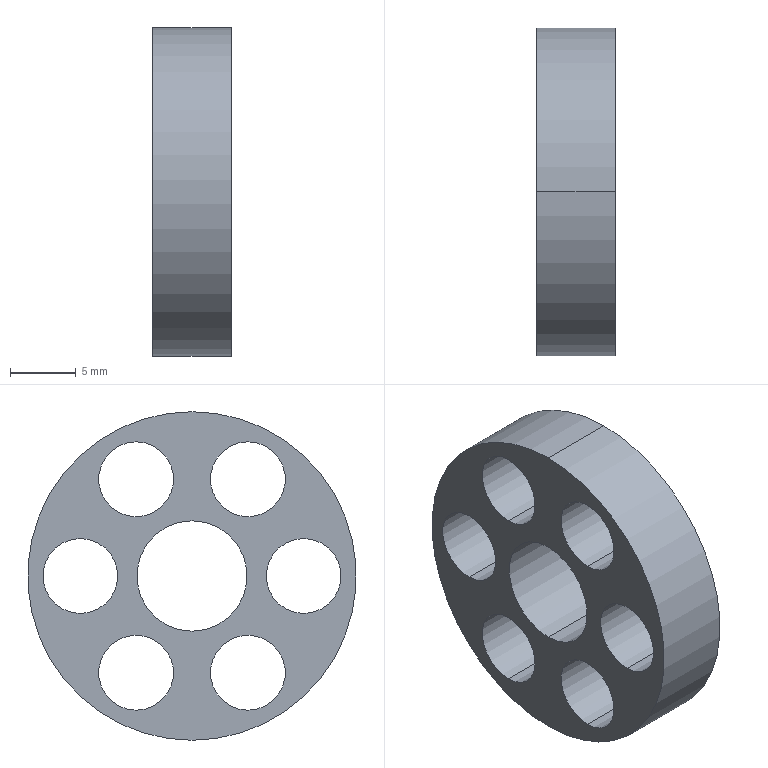Part | SolidWorks | features BaseBody 1 | 1 solid | 18 faces | box 6 x 25 x 25 mm | volume 1694 mm3 | cylinder 16 | plane 2 | commonest cylinder face diameters 5.7 x12 8.4 x2 25 x2
STEP:
#1=CARTESIAN_POINT('',(-3.,0.,-12.5));
#2=VERTEX_POINT('',#1);
#3=CARTESIAN_POINT('',(-3.,0.,12.5));
#4=VERTEX_POINT('',#3);
#5=CARTESIAN_POINT('',(-3.,0.,0.));
#6=DIRECTION('',(1.,0.,0.));
#7=DIRECTION('',(0.,0.,-1.));
#8=AXIS2_PLACEMENT_3D('',#5,#6,#7);
#9=CIRCLE('',#8,12.5);
#10=EDGE_CURVE('',#2,#4,#9,.T.);
#11=ORIENTED_EDGE('',*,*,#10,.T.);
#12=CARTESIAN_POINT('',(3.,0.,12.5));
#13=VERTEX_POINT('',#12);
#14=CARTESIAN_POINT('',(-3.,0.,12.5));
#15=DIRECTION('',(1.,0.,0.));
#16=VECTOR('',#15,1000.);
#17=LINE('',#14,#16);
#18=EDGE_CURVE('',#4,#13,#17,.T.);
#19=ORIENTED_EDGE('',*,*,#18,.T.);
#20=CARTESIAN_POINT('',(3.,0.,-12.5));
#21=VERTEX_POINT('',#20);
#22=CARTESIAN_POINT('',(3.,0.,0.));
#23=DIRECTION('',(-1.,0.,0.));
#24=DIRECTION('',(0.,0.,-1.));
#25=AXIS2_PLACEMENT_3D('',#22,#23,#24);
#26=CIRCLE('',#25,12.5);
#27=EDGE_CURVE('',#13,#21,#26,.T.);
#28=ORIENTED_EDGE('',*,*,#27,.T.);
#29=CARTESIAN_POINT('',(-3.,0.,-12.5));
#30=DIRECTION('',(1.,0.,0.));
#31=VECTOR('',#30,1000.);
#32=LINE('',#29,#31);
#33=EDGE_CURVE('',#2,#21,#32,.T.);
#34=ORIENTED_EDGE('',*,*,#33,.F.);
#35=EDGE_LOOP('',(#11,#19,#28,#34));
#36=FACE_OUTER_BOUND('',#35,.T.);
#37=CARTESIAN_POINT('',(-3.,0.,0.));
#38=DIRECTION('',(1.,0.,0.));
#39=DIRECTION('',(0.,0.,-1.));
#40=AXIS2_PLACEMENT_3D('',#37,#38,#39);
#41=CYLINDRICAL_SURFACE('',#40,12.5);
#42=ADVANCED_FACE('',(#36),#41,.T.);
#43=CARTESIAN_POINT('',(-3.,8.5,-2.85));
#44=VERTEX_POINT('',#43);
#45=CARTESIAN_POINT('',(-3.,8.5,2.85));
#46=VERTEX_POINT('',#45);
#47=CARTESIAN_POINT('',(-3.,8.5,0.));
#48=DIRECTION('',(-1.,0.,0.));
#49=DIRECTION('',(0.,0.,-1.));
#50=AXIS2_PLACEMENT_3D('',#47,#48,#49);
#51=CIRCLE('',#50,2.85);
#52=EDGE_CURVE('',#44,#46,#51,.T.);
#53=ORIENTED_EDGE('',*,*,#52,.T.);
#54=CARTESIAN_POINT('',(3.,8.5,2.85));
#55=VERTEX_POINT('',#54);
#56=CARTESIAN_POINT('',(-4.,8.5,2.85));
#57=DIRECTION('',(1.,0.,0.));
#58=VECTOR('',#57,1000.);
#59=LINE('',#56,#58);
#60=EDGE_CURVE('',#46,#55,#59,.T.);
#61=ORIENTED_EDGE('',*,*,#60,.T.);
#62=CARTESIAN_POINT('',(3.,8.5,-2.85));
#63=VERTEX_POINT('',#62);
#64=CARTESIAN_POINT('',(3.,8.5,0.));
#65=DIRECTION('',(-1.,0.,0.));
#66=DIRECTION('',(0.,0.,-1.));
#67=AXIS2_PLACEMENT_3D('',#64,#65,#66);
#68=CIRCLE('',#67,2.85);
#69=EDGE_CURVE('',#63,#55,#68,.T.);
#70=ORIENTED_EDGE('',*,*,#69,.F.);
#71=CARTESIAN_POINT('',(-4.,8.5,-2.85));
#72=DIRECTION('',(1.,0.,0.));
#73=VECTOR('',#72,1000.);
#74=LINE('',#71,#73);
#75=EDGE_CURVE('',#44,#63,#74,.T.);
#76=ORIENTED_EDGE('',*,*,#75,.F.);
#77=EDGE_LOOP('',(#53,#61,#70,#76));
#78=FACE_OUTER_BOUND('',#77,.T.);
#79=CARTESIAN_POINT('',(-4.,8.5,0.));
#80=DIRECTION('',(1.,0.,0.));
#81=DIRECTION('',(0.,0.,-1.));
#82=AXIS2_PLACEMENT_3D('',#79,#80,#81);
#83=CYLINDRICAL_SURFACE('',#82,2.85);
#84=ADVANCED_FACE('',(#78),#83,.F.);
#85=CARTESIAN_POINT('',(-3.,4.25,-10.211));
#86=VERTEX_POINT('',#85);
#87=CARTESIAN_POINT('',(-3.,4.25,-4.511));
#88=VERTEX_POINT('',#87);
#89=CARTESIAN_POINT('',(-3.,4.25,-7.361));
#90=DIRECTION('',(-1.,0.,0.));
#91=DIRECTION('',(0.,0.,-1.));
#92=AXIS2_PLACEMENT_3D('',#89,#90,#91);
#93=CIRCLE('',#92,2.85);
#94=EDGE_CURVE('',#86,#88,#93,.T.);
#95=ORIENTED_EDGE('',*,*,#94,.T.);
#96=CARTESIAN_POINT('',(3.,4.25,-4.511));
#97=VERTEX_POINT('',#96);
#98=CARTESIAN_POINT('',(-4.,4.25,-4.511));
#99=DIRECTION('',(1.,0.,0.));
#100=VECTOR('',#99,1000.);
#101=LINE('',#98,#100);
#102=EDGE_CURVE('',#88,#97,#101,.T.);
#103=ORIENTED_EDGE('',*,*,#102,.T.);
#104=CARTESIAN_POINT('',(3.,4.25,-10.211));
#105=VERTEX_POINT('',#104);
#106=CARTESIAN_POINT('',(3.,4.25,-7.361));
#107=DIRECTION('',(-1.,0.,0.));
#108=DIRECTION('',(0.,0.,-1.));
#109=AXIS2_PLACEMENT_3D('',#106,#107,#108);
#110=CIRCLE('',#109,2.85);
#111=EDGE_CURVE('',#105,#97,#110,.T.);
#112=ORIENTED_EDGE('',*,*,#111,.F.);
#113=CARTESIAN_POINT('',(-4.,4.25,-10.211));
#114=DIRECTION('',(1.,0.,0.));
#115=VECTOR('',#114,1000.);
#116=LINE('',#113,#115);
#117=EDGE_CURVE('',#86,#105,#116,.T.);
#118=ORIENTED_EDGE('',*,*,#117,.F.);
#119=EDGE_LOOP('',(#95,#103,#112,#118));
#120=FACE_OUTER_BOUND('',#119,.T.);
#121=CARTESIAN_POINT('',(-4.,4.25,-7.361));
#122=DIRECTION('',(1.,0.,0.));
#123=DIRECTION('',(0.,0.,-1.));
#124=AXIS2_PLACEMENT_3D('',#121,#122,#123);
#125=CYLINDRICAL_SURFACE('',#124,2.85);
#126=ADVANCED_FACE('',(#120),#125,.F.);
#127=CARTESIAN_POINT('',(-3.,0.,-4.2));
#128=VERTEX_POINT('',#127);
#129=CARTESIAN_POINT('',(-3.,0.,4.2));
#130=VERTEX_POINT('',#129);
#131=CARTESIAN_POINT('',(-3.,0.,0.));
#132=DIRECTION('',(-1.,0.,0.));
#133=DIRECTION('',(0.,0.,-1.));
#134=AXIS2_PLACEMENT_3D('',#131,#132,#133);
#135=CIRCLE('',#134,4.2);
#136=EDGE_CURVE('',#128,#130,#135,.T.);
#137=ORIENTED_EDGE('',*,*,#136,.T.);
#138=CARTESIAN_POINT('',(3.,0.,4.2));
#139=VERTEX_POINT('',#138);
#140=CARTESIAN_POINT('',(-4.,0.,4.2));
#141=DIRECTION('',(1.,0.,0.));
#142=VECTOR('',#141,1000.);
#143=LINE('',#140,#142);
#144=EDGE_CURVE('',#130,#139,#143,.T.);
#145=ORIENTED_EDGE('',*,*,#144,.T.);
#146=CARTESIAN_POINT('',(3.,0.,-4.2));
#147=VERTEX_POINT('',#146);
#148=CARTESIAN_POINT('',(3.,0.,0.));
#149=DIRECTION('',(-1.,0.,0.));
#150=DIRECTION('',(0.,0.,-1.));
#151=AXIS2_PLACEMENT_3D('',#148,#149,#150);
#152=CIRCLE('',#151,4.2);
#153=EDGE_CURVE('',#147,#139,#152,.T.);
#154=ORIENTED_EDGE('',*,*,#153,.F.);
#155=CARTESIAN_POINT('',(-4.,0.,-4.2));
#156=DIRECTION('',(1.,0.,0.));
#157=VECTOR('',#156,1000.);
#158=LINE('',#155,#157);
#159=EDGE_CURVE('',#128,#147,#158,.T.);
#160=ORIENTED_EDGE('',*,*,#159,.F.);
#161=EDGE_LOOP('',(#137,#145,#154,#160));
#162=FACE_OUTER_BOUND('',#161,.T.);
#163=CARTESIAN_POINT('',(-4.,0.,0.));
#164=DIRECTION('',(1.,0.,0.));
#165=DIRECTION('',(0.,0.,-1.));
#166=AXIS2_PLACEMENT_3D('',#163,#164,#165);
#167=CYLINDRICAL_SURFACE('',#166,4.2);
#168=ADVANCED_FACE('',(#162),#167,.F.);
#169=CARTESIAN_POINT('',(-3.,4.25,4.511));
#170=VERTEX_POINT('',#169);
#171=CARTESIAN_POINT('',(-3.,4.25,10.211));
#172=VERTEX_POINT('',#171);
#173=CARTESIAN_POINT('',(-3.,4.25,7.361));
#174=DIRECTION('',(-1.,0.,0.));
#175=DIRECTION('',(0.,0.,-1.));
#176=AXIS2_PLACEMENT_3D('',#173,#174,#175);
#177=CIRCLE('',#176,2.85);
#178=EDGE_CURVE('',#170,#172,#177,.T.);
#179=ORIENTED_EDGE('',*,*,#178,.T.);
#180=CARTESIAN_POINT('',(3.,4.25,10.211));
#181=VERTEX_POINT('',#180);
#182=CARTESIAN_POINT('',(-4.,4.25,10.211));
#183=DIRECTION('',(1.,0.,0.));
#184=VECTOR('',#183,1000.);
#185=LINE('',#182,#184);
#186=EDGE_CURVE('',#172,#181,#185,.T.);
#187=ORIENTED_EDGE('',*,*,#186,.T.);
#188=CARTESIAN_POINT('',(3.,4.25,4.511));
#189=VERTEX_POINT('',#188);
#190=CARTESIAN_POINT('',(3.,4.25,7.361));
#191=DIRECTION('',(-1.,0.,0.));
#192=DIRECTION('',(0.,0.,-1.));
#193=AXIS2_PLACEMENT_3D('',#190,#191,#192);
#194=CIRCLE('',#193,2.85);
#195=EDGE_CURVE('',#189,#181,#194,.T.);
#196=ORIENTED_EDGE('',*,*,#195,.F.);
#197=CARTESIAN_POINT('',(-4.,4.25,4.511));
#198=DIRECTION('',(1.,0.,0.));
#199=VECTOR('',#198,1000.);
#200=LINE('',#197,#199);
#201=EDGE_CURVE('',#170,#189,#200,.T.);
#202=ORIENTED_EDGE('',*,*,#201,.F.);
#203=EDGE_LOOP('',(#179,#187,#196,#202));
#204=FACE_OUTER_BOUND('',#203,.T.);
#205=CARTESIAN_POINT('',(-4.,4.25,7.361));
#206=DIRECTION('',(1.,0.,0.));
#207=DIRECTION('',(0.,0.,-1.));
#208=AXIS2_PLACEMENT_3D('',#205,#206,#207);
#209=CYLINDRICAL_SURFACE('',#208,2.85);
#210=ADVANCED_FACE('',(#204),#209,.F.);
#211=CARTESIAN_POINT('',(-3.,-4.25,-10.211));
#212=VERTEX_POINT('',#211);
#213=CARTESIAN_POINT('',(-3.,-4.25,-4.511));
#214=VERTEX_POINT('',#213);
#215=CARTESIAN_POINT('',(-3.,-4.25,-7.361));
#216=DIRECTION('',(-1.,0.,0.));
#217=DIRECTION('',(0.,0.,-1.));
#218=AXIS2_PLACEMENT_3D('',#215,#216,#217);
#219=CIRCLE('',#218,2.85);
#220=EDGE_CURVE('',#212,#214,#219,.T.);
#221=ORIENTED_EDGE('',*,*,#220,.T.);
#222=CARTESIAN_POINT('',(3.,-4.25,-4.511));
#223=VERTEX_POINT('',#222);
#224=CARTESIAN_POINT('',(-4.,-4.25,-4.511));
#225=DIRECTION('',(1.,0.,0.));
#226=VECTOR('',#225,1000.);
#227=LINE('',#224,#226);
#228=EDGE_CURVE('',#214,#223,#227,.T.);
#229=ORIENTED_EDGE('',*,*,#228,.T.);
#230=CARTESIAN_POINT('',(3.,-4.25,-10.211));
#231=VERTEX_POINT('',#230);
#232=CARTESIAN_POINT('',(3.,-4.25,-7.361));
#233=DIRECTION('',(-1.,0.,0.));
#234=DIRECTION('',(0.,0.,-1.));
#235=AXIS2_PLACEMENT_3D('',#232,#233,#234);
#236=CIRCLE('',#235,2.85);
#237=EDGE_CURVE('',#231,#223,#236,.T.);
#238=ORIENTED_EDGE('',*,*,#237,.F.);
#239=CARTESIAN_POINT('',(-4.,-4.25,-10.211));
#240=DIRECTION('',(1.,0.,0.));
#241=VECTOR('',#240,1000.);
#242=LINE('',#239,#241);
#243=EDGE_CURVE('',#212,#231,#242,.T.);
#244=ORIENTED_EDGE('',*,*,#243,.F.);
#245=EDGE_LOOP('',(#221,#229,#238,#244));
#246=FACE_OUTER_BOUND('',#245,.T.);
#247=CARTESIAN_POINT('',(-4.,-4.25,-7.361));
#248=DIRECTION('',(1.,0.,0.));
#249=DIRECTION('',(0.,0.,-1.));
#250=AXIS2_PLACEMENT_3D('',#247,#248,#249);
#251=CYLINDRICAL_SURFACE('',#250,2.85);
#252=ADVANCED_FACE('',(#246),#251,.F.);
#253=CARTESIAN_POINT('',(-3.,-8.5,-2.85));
#254=VERTEX_POINT('',#253);
#255=CARTESIAN_POINT('',(-3.,-8.5,2.85));
#256=VERTEX_POINT('',#255);
#257=CARTESIAN_POINT('',(-3.,-8.5,0.));
#258=DIRECTION('',(-1.,0.,0.));
#259=DIRECTION('',(0.,0.,-1.));
#260=AXIS2_PLACEMENT_3D('',#257,#258,#259);
#261=CIRCLE('',#260,2.85);
#262=EDGE_CURVE('',#254,#256,#261,.T.);
#263=ORIENTED_EDGE('',*,*,#262,.T.);
#264=CARTESIAN_POINT('',(3.,-8.5,2.85));
#265=VERTEX_POINT('',#264);
#266=CARTESIAN_POINT('',(-4.,-8.5,2.85));
#267=DIRECTION('',(1.,0.,0.));
#268=VECTOR('',#267,1000.);
#269=LINE('',#266,#268);
#270=EDGE_CURVE('',#256,#265,#269,.T.);
#271=ORIENTED_EDGE('',*,*,#270,.T.);
#272=CARTESIAN_POINT('',(3.,-8.5,-2.85));
#273=VERTEX_POINT('',#272);
#274=CARTESIAN_POINT('',(3.,-8.5,0.));
#275=DIRECTION('',(-1.,0.,0.));
#276=DIRECTION('',(0.,0.,-1.));
#277=AXIS2_PLACEMENT_3D('',#274,#275,#276);
#278=CIRCLE('',#277,2.85);
#279=EDGE_CURVE('',#273,#265,#278,.T.);
#280=ORIENTED_EDGE('',*,*,#279,.F.);
#281=CARTESIAN_POINT('',(-4.,-8.5,-2.85));
#282=DIRECTION('',(1.,0.,0.));
#283=VECTOR('',#282,1000.);
#284=LINE('',#281,#283);
#285=EDGE_CURVE('',#254,#273,#284,.T.);
#286=ORIENTED_EDGE('',*,*,#285,.F.);
#287=EDGE_LOOP('',(#263,#271,#280,#286));
#288=FACE_OUTER_BOUND('',#287,.T.);
#289=CARTESIAN_POINT('',(-4.,-8.5,0.));
#290=DIRECTION('',(1.,0.,0.));
#291=DIRECTION('',(0.,0.,-1.));
#292=AXIS2_PLACEMENT_3D('',#289,#290,#291);
#293=CYLINDRICAL_SURFACE('',#292,2.85);
#294=ADVANCED_FACE('',(#288),#293,.F.);
#295=CARTESIAN_POINT('',(-3.,-4.25,4.511));
#296=VERTEX_POINT('',#295);
#297=CARTESIAN_POINT('',(-3.,-4.25,10.211));
#298=VERTEX_POINT('',#297);
#299=CARTESIAN_POINT('',(-3.,-4.25,7.361));
#300=DIRECTION('',(-1.,0.,0.));
#301=DIRECTION('',(0.,0.,-1.));
#302=AXIS2_PLACEMENT_3D('',#299,#300,#301);
#303=CIRCLE('',#302,2.85);
#304=EDGE_CURVE('',#296,#298,#303,.T.);
#305=ORIENTED_EDGE('',*,*,#304,.T.);
#306=CARTESIAN_POINT('',(3.,-4.25,10.211));
#307=VERTEX_POINT('',#306);
#308=CARTESIAN_POINT('',(-4.,-4.25,10.211));
#309=DIRECTION('',(1.,0.,0.));
#310=VECTOR('',#309,1000.);
#311=LINE('',#308,#310);
#312=EDGE_CURVE('',#298,#307,#311,.T.);
#313=ORIENTED_EDGE('',*,*,#312,.T.);
#314=CARTESIAN_POINT('',(3.,-4.25,4.511));
#315=VERTEX_POINT('',#314);
#316=CARTESIAN_POINT('',(3.,-4.25,7.361));
#317=DIRECTION('',(-1.,0.,0.));
#318=DIRECTION('',(0.,0.,-1.));
#319=AXIS2_PLACEMENT_3D('',#316,#317,#318);
#320=CIRCLE('',#319,2.85);
#321=EDGE_CURVE('',#315,#307,#320,.T.);
#322=ORIENTED_EDGE('',*,*,#321,.F.);
#323=CARTESIAN_POINT('',(-4.,-4.25,4.511));
#324=DIRECTION('',(1.,0.,0.));
#325=VECTOR('',#324,1000.);
#326=LINE('',#323,#325);
#327=EDGE_CURVE('',#296,#315,#326,.T.);
#328=ORIENTED_EDGE('',*,*,#327,.F.);
#329=EDGE_LOOP('',(#305,#313,#322,#328));
#330=FACE_OUTER_BOUND('',#329,.T.);
#331=CARTESIAN_POINT('',(-4.,-4.25,7.361));
#332=DIRECTION('',(1.,0.,0.));
#333=DIRECTION('',(0.,0.,-1.));
#334=AXIS2_PLACEMENT_3D('',#331,#332,#333);
#335=CYLINDRICAL_SURFACE('',#334,2.85);
#336=ADVANCED_FACE('',(#330),#335,.F.);
#337=ORIENTED_EDGE('',*,*,#18,.F.);
#338=CARTESIAN_POINT('',(-3.,0.,0.));
#339=DIRECTION('',(1.,0.,0.));
#340=DIRECTION('',(0.,0.,-1.));
#341=AXIS2_PLACEMENT_3D('',#338,#339,#340);
#342=CIRCLE('',#341,12.5);
#343=EDGE_CURVE('',#4,#2,#342,.T.);
#344=ORIENTED_EDGE('',*,*,#343,.T.);
#345=ORIENTED_EDGE('',*,*,#33,.T.);
#346=CARTESIAN_POINT('',(3.,0.,0.));
#347=DIRECTION('',(-1.,0.,0.));
#348=DIRECTION('',(0.,0.,-1.));
#349=AXIS2_PLACEMENT_3D('',#346,#347,#348);
#350=CIRCLE('',#349,12.5);
#351=EDGE_CURVE('',#21,#13,#350,.T.);
#352=ORIENTED_EDGE('',*,*,#351,.T.);
#353=EDGE_LOOP('',(#337,#344,#345,#352));
#354=FACE_OUTER_BOUND('',#353,.T.);
#355=CARTESIAN_POINT('',(-3.,0.,0.));
#356=DIRECTION('',(1.,0.,0.));
#357=DIRECTION('',(0.,0.,-1.));
#358=AXIS2_PLACEMENT_3D('',#355,#356,#357);
#359=CYLINDRICAL_SURFACE('',#358,12.5);
#360=ADVANCED_FACE('',(#354),#359,.T.);
#361=ORIENTED_EDGE('',*,*,#52,.F.);
#362=CARTESIAN_POINT('',(-3.,8.5,0.));
#363=DIRECTION('',(-1.,0.,0.));
#364=DIRECTION('',(0.,0.,-1.));
#365=AXIS2_PLACEMENT_3D('',#362,#363,#364);
#366=CIRCLE('',#365,2.85);
#367=EDGE_CURVE('',#46,#44,#366,.T.);
#368=ORIENTED_EDGE('',*,*,#367,.F.);
#369=EDGE_LOOP('',(#361,#368));
#370=FACE_BOUND('',#369,.T.);
#371=ORIENTED_EDGE('',*,*,#94,.F.);
#372=CARTESIAN_POINT('',(-3.,4.25,-7.361));
#373=DIRECTION('',(-1.,0.,0.));
#374=DIRECTION('',(0.,0.,-1.));
#375=AXIS2_PLACEMENT_3D('',#372,#373,#374);
#376=CIRCLE('',#375,2.85);
#377=EDGE_CURVE('',#88,#86,#376,.T.);
#378=ORIENTED_EDGE('',*,*,#377,.F.);
#379=EDGE_LOOP('',(#371,#378));
#380=FACE_BOUND('',#379,.T.);
#381=ORIENTED_EDGE('',*,*,#136,.F.);
#382=CARTESIAN_POINT('',(-3.,0.,0.));
#383=DIRECTION('',(-1.,0.,0.));
#384=DIRECTION('',(0.,0.,-1.));
#385=AXIS2_PLACEMENT_3D('',#382,#383,#384);
#386=CIRCLE('',#385,4.2);
#387=EDGE_CURVE('',#130,#128,#386,.T.);
#388=ORIENTED_EDGE('',*,*,#387,.F.);
#389=EDGE_LOOP('',(#381,#388));
#390=FACE_BOUND('',#389,.T.);
#391=ORIENTED_EDGE('',*,*,#178,.F.);
#392=CARTESIAN_POINT('',(-3.,4.25,7.361));
#393=DIRECTION('',(-1.,0.,0.));
#394=DIRECTION('',(0.,0.,-1.));
#395=AXIS2_PLACEMENT_3D('',#392,#393,#394);
#396=CIRCLE('',#395,2.85);
#397=EDGE_CURVE('',#172,#170,#396,.T.);
#398=ORIENTED_EDGE('',*,*,#397,.F.);
#399=EDGE_LOOP('',(#391,#398));
#400=FACE_BOUND('',#399,.T.);
#401=ORIENTED_EDGE('',*,*,#220,.F.);
#402=CARTESIAN_POINT('',(-3.,-4.25,-7.361));
#403=DIRECTION('',(-1.,0.,0.));
#404=DIRECTION('',(0.,0.,-1.));
#405=AXIS2_PLACEMENT_3D('',#402,#403,#404);
#406=CIRCLE('',#405,2.85);
#407=EDGE_CURVE('',#214,#212,#406,.T.);
#408=ORIENTED_EDGE('',*,*,#407,.F.);
#409=EDGE_LOOP('',(#401,#408));
#410=FACE_BOUND('',#409,.T.);
#411=ORIENTED_EDGE('',*,*,#262,.F.);
#412=CARTESIAN_POINT('',(-3.,-8.5,0.));
#413=DIRECTION('',(-1.,0.,0.));
#414=DIRECTION('',(0.,0.,-1.));
#415=AXIS2_PLACEMENT_3D('',#412,#413,#414);
#416=CIRCLE('',#415,2.85);
#417=EDGE_CURVE('',#256,#254,#416,.T.);
#418=ORIENTED_EDGE('',*,*,#417,.F.);
#419=EDGE_LOOP('',(#411,#418));
#420=FACE_BOUND('',#419,.T.);
#421=ORIENTED_EDGE('',*,*,#304,.F.);
#422=CARTESIAN_POINT('',(-3.,-4.25,7.361));
#423=DIRECTION('',(-1.,0.,0.));
#424=DIRECTION('',(0.,0.,-1.));
#425=AXIS2_PLACEMENT_3D('',#422,#423,#424);
#426=CIRCLE('',#425,2.85);
#427=EDGE_CURVE('',#298,#296,#426,.T.);
#428=ORIENTED_EDGE('',*,*,#427,.F.);
#429=EDGE_LOOP('',(#421,#428));
#430=FACE_BOUND('',#429,.T.);
#431=ORIENTED_EDGE('',*,*,#10,.F.);
#432=ORIENTED_EDGE('',*,*,#343,.F.);
#433=EDGE_LOOP('',(#431,#432));
#434=FACE_OUTER_BOUND('',#433,.T.);
#435=CARTESIAN_POINT('',(-3.,0.,0.));
#436=DIRECTION('',(1.,0.,0.));
#437=DIRECTION('',(0.,0.,-1.));
#438=AXIS2_PLACEMENT_3D('',#435,#436,#437);
#439=PLANE('',#438);
#440=ADVANCED_FACE('',(#370,#380,#390,#400,#410,#420,#430,#434),#439,.F.);
#441=ORIENTED_EDGE('',*,*,#69,.T.);
#442=CARTESIAN_POINT('',(3.,8.5,0.));
#443=DIRECTION('',(-1.,0.,0.));
#444=DIRECTION('',(0.,0.,-1.));
#445=AXIS2_PLACEMENT_3D('',#442,#443,#444);
#446=CIRCLE('',#445,2.85);
#447=EDGE_CURVE('',#55,#63,#446,.T.);
#448=ORIENTED_EDGE('',*,*,#447,.T.);
#449=EDGE_LOOP('',(#441,#448));
#450=FACE_BOUND('',#449,.T.);
#451=ORIENTED_EDGE('',*,*,#111,.T.);
#452=CARTESIAN_POINT('',(3.,4.25,-7.361));
#453=DIRECTION('',(-1.,0.,0.));
#454=DIRECTION('',(0.,0.,-1.));
#455=AXIS2_PLACEMENT_3D('',#452,#453,#454);
#456=CIRCLE('',#455,2.85);
#457=EDGE_CURVE('',#97,#105,#456,.T.);
#458=ORIENTED_EDGE('',*,*,#457,.T.);
#459=EDGE_LOOP('',(#451,#458));
#460=FACE_BOUND('',#459,.T.);
#461=ORIENTED_EDGE('',*,*,#153,.T.);
#462=CARTESIAN_POINT('',(3.,0.,0.));
#463=DIRECTION('',(-1.,0.,0.));
#464=DIRECTION('',(0.,0.,-1.));
#465=AXIS2_PLACEMENT_3D('',#462,#463,#464);
#466=CIRCLE('',#465,4.2);
#467=EDGE_CURVE('',#139,#147,#466,.T.);
#468=ORIENTED_EDGE('',*,*,#467,.T.);
#469=EDGE_LOOP('',(#461,#468));
#470=FACE_BOUND('',#469,.T.);
#471=ORIENTED_EDGE('',*,*,#195,.T.);
#472=CARTESIAN_POINT('',(3.,4.25,7.361));
#473=DIRECTION('',(-1.,0.,0.));
#474=DIRECTION('',(0.,0.,-1.));
#475=AXIS2_PLACEMENT_3D('',#472,#473,#474);
#476=CIRCLE('',#475,2.85);
#477=EDGE_CURVE('',#181,#189,#476,.T.);
#478=ORIENTED_EDGE('',*,*,#477,.T.);
#479=EDGE_LOOP('',(#471,#478));
#480=FACE_BOUND('',#479,.T.);
#481=ORIENTED_EDGE('',*,*,#237,.T.);
#482=CARTESIAN_POINT('',(3.,-4.25,-7.361));
#483=DIRECTION('',(-1.,0.,0.));
#484=DIRECTION('',(0.,0.,-1.));
#485=AXIS2_PLACEMENT_3D('',#482,#483,#484);
#486=CIRCLE('',#485,2.85);
#487=EDGE_CURVE('',#223,#231,#486,.T.);
#488=ORIENTED_EDGE('',*,*,#487,.T.);
#489=EDGE_LOOP('',(#481,#488));
#490=FACE_BOUND('',#489,.T.);
#491=ORIENTED_EDGE('',*,*,#279,.T.);
#492=CARTESIAN_POINT('',(3.,-8.5,0.));
#493=DIRECTION('',(-1.,0.,0.));
#494=DIRECTION('',(0.,0.,-1.));
#495=AXIS2_PLACEMENT_3D('',#492,#493,#494);
#496=CIRCLE('',#495,2.85);
#497=EDGE_CURVE('',#265,#273,#496,.T.);
#498=ORIENTED_EDGE('',*,*,#497,.T.);
#499=EDGE_LOOP('',(#491,#498));
#500=FACE_BOUND('',#499,.T.);
#501=ORIENTED_EDGE('',*,*,#321,.T.);
#502=CARTESIAN_POINT('',(3.,-4.25,7.361));
#503=DIRECTION('',(-1.,0.,0.));
#504=DIRECTION('',(0.,0.,-1.));
#505=AXIS2_PLACEMENT_3D('',#502,#503,#504);
#506=CIRCLE('',#505,2.85);
#507=EDGE_CURVE('',#307,#315,#506,.T.);
#508=ORIENTED_EDGE('',*,*,#507,.T.);
#509=EDGE_LOOP('',(#501,#508));
#510=FACE_BOUND('',#509,.T.);
#511=ORIENTED_EDGE('',*,*,#351,.F.);
#512=ORIENTED_EDGE('',*,*,#27,.F.);
#513=EDGE_LOOP('',(#511,#512));
#514=FACE_OUTER_BOUND('',#513,.T.);
#515=CARTESIAN_POINT('',(3.,0.,0.));
#516=DIRECTION('',(1.,0.,0.));
#517=DIRECTION('',(0.,0.,-1.));
#518=AXIS2_PLACEMENT_3D('',#515,#516,#517);
#519=PLANE('',#518);
#520=ADVANCED_FACE('',(#450,#460,#470,#480,#490,#500,#510,#514),#519,.T.);
#521=ORIENTED_EDGE('',*,*,#60,.F.);
#522=ORIENTED_EDGE('',*,*,#367,.T.);
#523=ORIENTED_EDGE('',*,*,#75,.T.);
#524=ORIENTED_EDGE('',*,*,#447,.F.);
#525=EDGE_LOOP('',(#521,#522,#523,#524));
#526=FACE_OUTER_BOUND('',#525,.T.);
#527=CARTESIAN_POINT('',(-4.,8.5,0.));
#528=DIRECTION('',(1.,0.,0.));
#529=DIRECTION('',(0.,0.,-1.));
#530=AXIS2_PLACEMENT_3D('',#527,#528,#529);
#531=CYLINDRICAL_SURFACE('',#530,2.85);
#532=ADVANCED_FACE('',(#526),#531,.F.);
#533=ORIENTED_EDGE('',*,*,#102,.F.);
#534=ORIENTED_EDGE('',*,*,#377,.T.);
#535=ORIENTED_EDGE('',*,*,#117,.T.);
#536=ORIENTED_EDGE('',*,*,#457,.F.);
#537=EDGE_LOOP('',(#533,#534,#535,#536));
#538=FACE_OUTER_BOUND('',#537,.T.);
#539=CARTESIAN_POINT('',(-4.,4.25,-7.361));
#540=DIRECTION('',(1.,0.,0.));
#541=DIRECTION('',(0.,0.,-1.));
#542=AXIS2_PLACEMENT_3D('',#539,#540,#541);
#543=CYLINDRICAL_SURFACE('',#542,2.85);
#544=ADVANCED_FACE('',(#538),#543,.F.);
#545=ORIENTED_EDGE('',*,*,#144,.F.);
#546=ORIENTED_EDGE('',*,*,#387,.T.);
#547=ORIENTED_EDGE('',*,*,#159,.T.);
#548=ORIENTED_EDGE('',*,*,#467,.F.);
#549=EDGE_LOOP('',(#545,#546,#547,#548));
#550=FACE_OUTER_BOUND('',#549,.T.);
#551=CARTESIAN_POINT('',(-4.,0.,0.));
#552=DIRECTION('',(1.,0.,0.));
#553=DIRECTION('',(0.,0.,-1.));
#554=AXIS2_PLACEMENT_3D('',#551,#552,#553);
#555=CYLINDRICAL_SURFACE('',#554,4.2);
#556=ADVANCED_FACE('',(#550),#555,.F.);
#557=ORIENTED_EDGE('',*,*,#186,.F.);
#558=ORIENTED_EDGE('',*,*,#397,.T.);
#559=ORIENTED_EDGE('',*,*,#201,.T.);
#560=ORIENTED_EDGE('',*,*,#477,.F.);
#561=EDGE_LOOP('',(#557,#558,#559,#560));
#562=FACE_OUTER_BOUND('',#561,.T.);
#563=CARTESIAN_POINT('',(-4.,4.25,7.361));
#564=DIRECTION('',(1.,0.,0.));
#565=DIRECTION('',(0.,0.,-1.));
#566=AXIS2_PLACEMENT_3D('',#563,#564,#565);
#567=CYLINDRICAL_SURFACE('',#566,2.85);
#568=ADVANCED_FACE('',(#562),#567,.F.);
#569=ORIENTED_EDGE('',*,*,#228,.F.);
#570=ORIENTED_EDGE('',*,*,#407,.T.);
#571=ORIENTED_EDGE('',*,*,#243,.T.);
#572=ORIENTED_EDGE('',*,*,#487,.F.);
#573=EDGE_LOOP('',(#569,#570,#571,#572));
#574=FACE_OUTER_BOUND('',#573,.T.);
#575=CARTESIAN_POINT('',(-4.,-4.25,-7.361));
#576=DIRECTION('',(1.,0.,0.));
#577=DIRECTION('',(0.,0.,-1.));
#578=AXIS2_PLACEMENT_3D('',#575,#576,#577);
#579=CYLINDRICAL_SURFACE('',#578,2.85);
#580=ADVANCED_FACE('',(#574),#579,.F.);
#581=ORIENTED_EDGE('',*,*,#270,.F.);
#582=ORIENTED_EDGE('',*,*,#417,.T.);
#583=ORIENTED_EDGE('',*,*,#285,.T.);
#584=ORIENTED_EDGE('',*,*,#497,.F.);
#585=EDGE_LOOP('',(#581,#582,#583,#584));
#586=FACE_OUTER_BOUND('',#585,.T.);
#587=CARTESIAN_POINT('',(-4.,-8.5,0.));
#588=DIRECTION('',(1.,0.,0.));
#589=DIRECTION('',(0.,0.,-1.));
#590=AXIS2_PLACEMENT_3D('',#587,#588,#589);
#591=CYLINDRICAL_SURFACE('',#590,2.85);
#592=ADVANCED_FACE('',(#586),#591,.F.);
#593=ORIENTED_EDGE('',*,*,#312,.F.);
#594=ORIENTED_EDGE('',*,*,#427,.T.);
#595=ORIENTED_EDGE('',*,*,#327,.T.);
#596=ORIENTED_EDGE('',*,*,#507,.F.);
#597=EDGE_LOOP('',(#593,#594,#595,#596));
#598=FACE_OUTER_BOUND('',#597,.T.);
#599=CARTESIAN_POINT('',(-4.,-4.25,7.361));
#600=DIRECTION('',(1.,0.,0.));
#601=DIRECTION('',(0.,0.,-1.));
#602=AXIS2_PLACEMENT_3D('',#599,#600,#601);
#603=CYLINDRICAL_SURFACE('',#602,2.85);
#604=ADVANCED_FACE('',(#598),#603,.F.);
#605=CLOSED_SHELL('',(#42,#84,#126,#168,#210,#252,#294,#336,#360,#440,#520,#532,#544,#556,#568,#580,#592,#604));
#606=MANIFOLD_SOLID_BREP('',#605);
#607=CARTESIAN_POINT('',(0.,0.,0.));
#608=DIRECTION('',(0.,0.,1.));
#609=DIRECTION('',(1.,0.,0.));
#610=AXIS2_PLACEMENT_3D('',#607,#608,#609);
#611=(LENGTH_UNIT()NAMED_UNIT(*)SI_UNIT(.MILLI.,.METRE.));
#612=UNCERTAINTY_MEASURE_WITH_UNIT(LENGTH_MEASURE(0.00001),#611,'','');
#613=(NAMED_UNIT(*)PLANE_ANGLE_UNIT()SI_UNIT($,.RADIAN.));
#614=(NAMED_UNIT(*)SI_UNIT($,.STERADIAN.)SOLID_ANGLE_UNIT());
#615=(GEOMETRIC_REPRESENTATION_CONTEXT(3)GLOBAL_UNCERTAINTY_ASSIGNED_CONTEXT((#612))GLOBAL_UNIT_ASSIGNED_CONTEXT((#611,#613,#614))REPRESENTATION_CONTEXT('',''));
#616=ADVANCED_BREP_SHAPE_REPRESENTATION('',(#606,#610),#615);